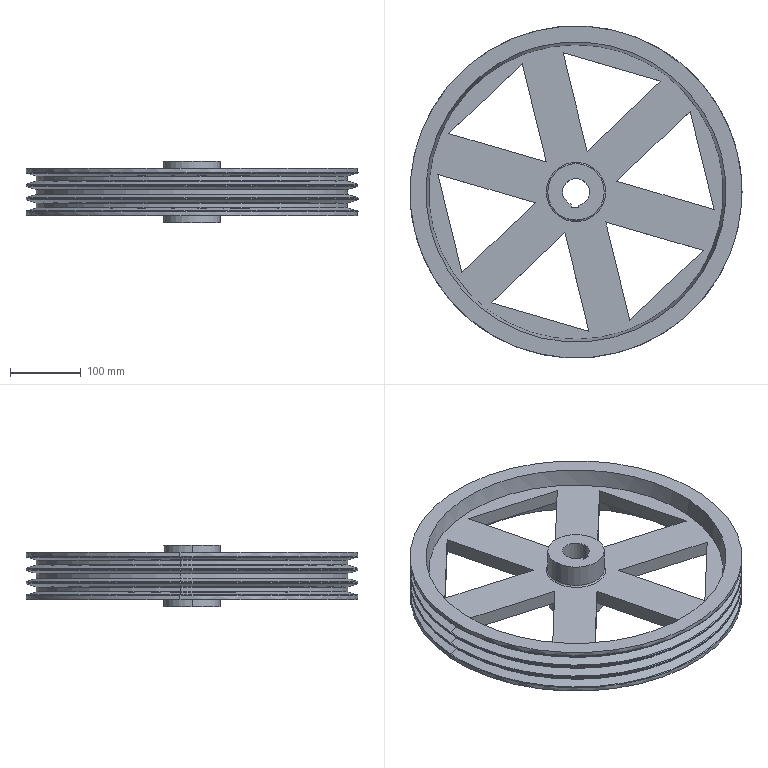Part | SolidWorks | features ICE 5, Fillet 4, BaseBody 1, RevCut 1 | 1 solid | 90 faces | box 470 x 470 x 87 mm | volume 3518075 mm3 | plane 27 | torus 26 | cylinder 21 | cone 16 | commonest cylinder face diameters 470 x8 441.4 x6 80 x4 38 x3